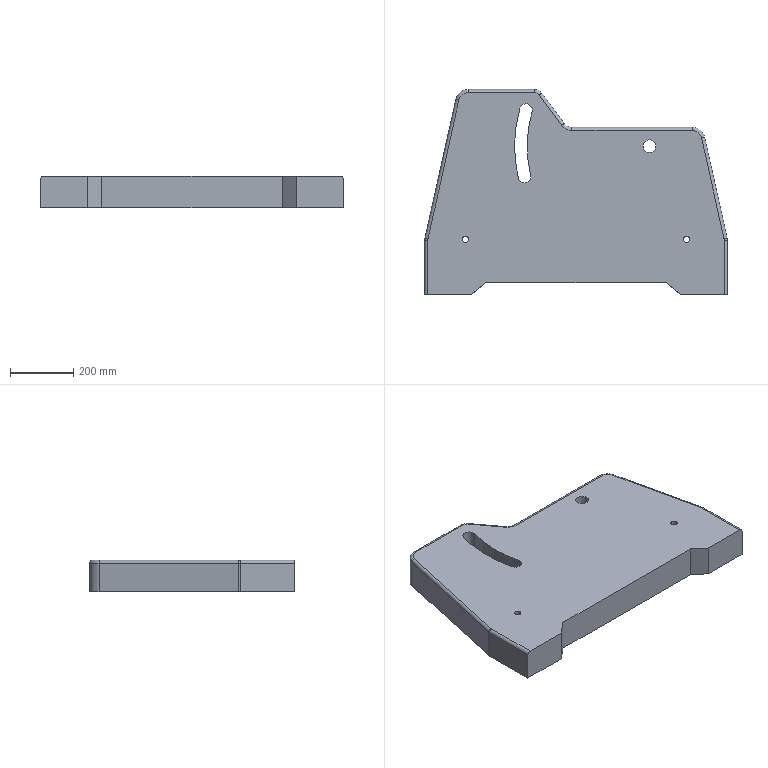Part | Creo | features CURVE 6, PROTRUSION 4, DATUM PLANE 3, ROUND 3, COORDINATE SYSTEM 1, CUT 1 | 1 solid | 63 faces | box 960 x 650 x 100 mm | volume 16944172 mm3 | plane 29 | cylinder 28 | torus 6 | commonest cylinder face diameters 20 x11 40 x4 60 x4 80 x3 70 x2 745.84 x1